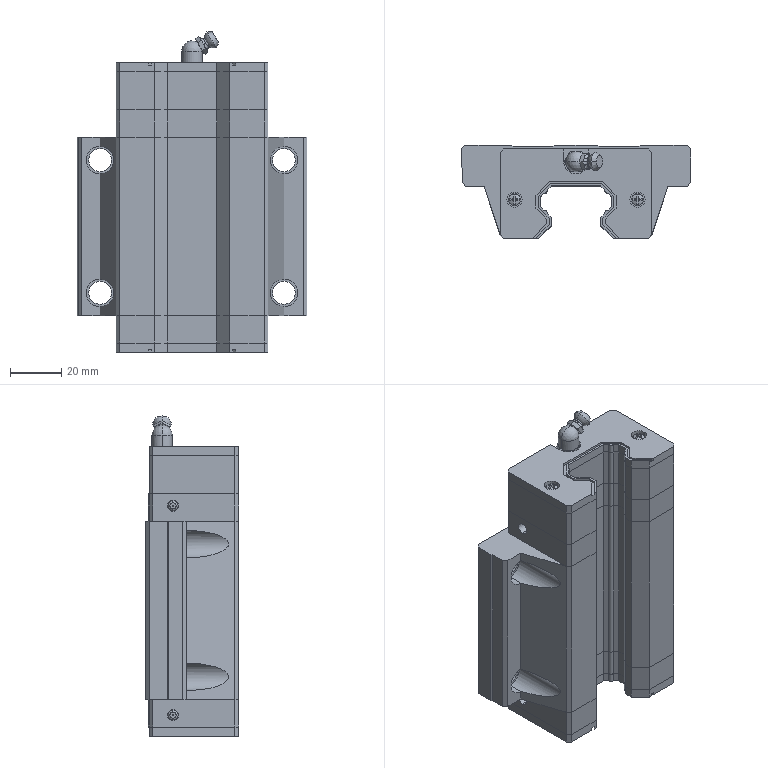Part | SolidWorks | features ICE 22, Extrusion 5, MirrorPattern 5, Fillet 4, MirrorSolid 4, Chamfer 3, RevCut 3, Dome 2, LPattern 2, Revolution 2, DeleteBody 1, LibraryFeature 1 | 7 solids | 475 faces | box 90 x 36.5 x 125.4 mm | volume 221238 mm3 | plane 323 | cylinder 94 | torus 25 | cone 23 | sphere 10 | commonest cylinder face diameters 2.822 x36 4.26 x12 0.575 x8 4.788 x8 5.985 x8 9 x8